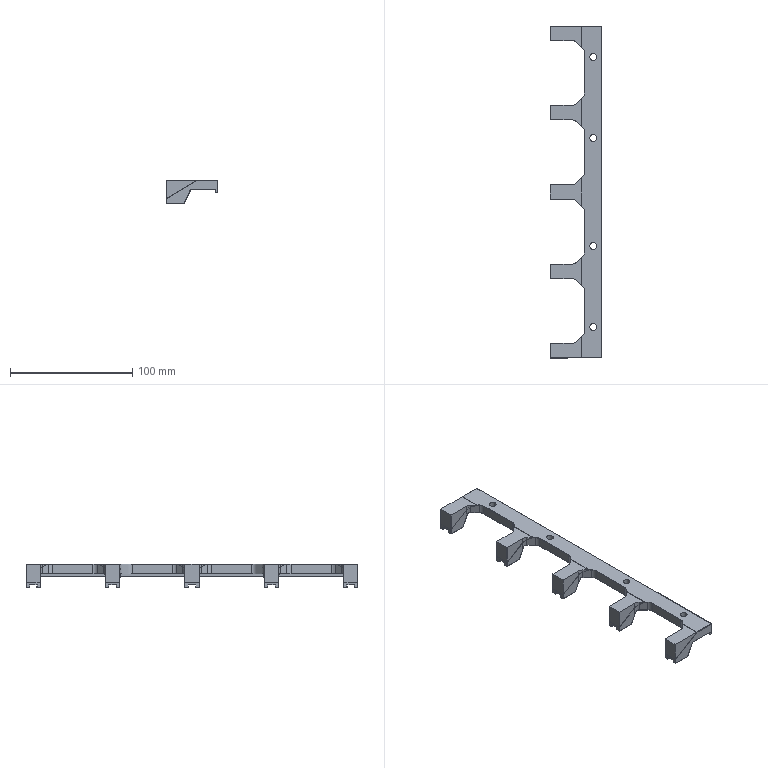CAM job | NX | 3+2 milling, drilling | part box 42 x 271.8 x 19 mm | stock box 45 x 277 x 25 mm
Tools:
number,name,description,diameter,corner_radius,flute_length,length,flutes
4,D4,平底铣刀-粗,4.0,0.0,25.0,75.0,2
6,D6,平底铣刀-粗,6.0,0.0,25.0,75.0,2
9,D10,平底铣刀-粗,10.0,0.0,35.0,75.0,2
7,D6-J,平底铣刀-精,6.0,0.0,25.0,75.0,2
10,D10-J,平底铣刀-精,10.0,0.0,35.0,75.0,2
18,D6R0.5,圆鼻刀-粗,6.0,0.5,50.0,75.0,2
1,D80R0.8飞刀,圆鼻刀-粗,80.0,0.8,50.0,75.0,2
2,D6倒角刀,倒角刀,6.0,0.0,3.0,25.0,2
17,钻头5.5,Twist Drill 5 mm,5.5,0.0,52.0,54.0,2
Operations:
program,operation,operation_type,tool,method,geometry_group,spindle_rpm,surface_speed,feed_per_tooth,feed_cut,feed_plunge,cut_length_mm,path_length_mm,cut_time_min,machine_time_min
C,型腔铣开粗-中_COPY_1,CavityMilling,D6,分层开粗-切深K-步距G,W-C,8000.0,150.796,0.1875,3000.0,100.0,19481.465,24446.704,6.494,7.228
C,等高精光往复爬面_COPY_1_COPY,ZLevelMilling,D6R0.5,等高爬面-切深K-步距G,W-C,7000.0,131.947,0.2857,4000.0,100.0,36709.228,37755.282,9.177,9.282
B,动态开粗D10_COPY_1,CavityMilling,D10,动态开粗-切深K-步距K,W-B,8000.0,251.32,0.25,4000.0,100.0,27133.852,27169.652,6.784,6.787
B,型腔铣开粗-中_COPY,CavityMilling,D10,分层开粗-切深K-步距G,W-B,8000.0,251.32,0.25,4000.0,100.0,20003.603,20348.798,5.001,5.05
B,底壁铣分层开粗-中_COPY,VolumeBased25DMillingOperation,D4,分层开粗-切深K-步距G,W-B,8000.0,100.528,0.125,2000.0,100.0,2370.316,2705.264,1.185,1.219
B,平面去毛刺6X45L_COPY,SurfaceContour,D6倒角刀,爬面_倒角-切深0-步距G,W-B,6500.0,122.519,0.1154,1500.0,100.0,1332.351,3197.122,0.8882,1.075
B,等高精光往复爬面_COPY,ZLevelMilling,D6R0.5,等高爬面-切深K-步距G,W-B,7000.0,131.947,0.2857,4000.0,100.0,12801.608,13764.402,3.2,3.297
B,底壁铣精光底面-中_COPY,VolumeBased25DMillingOperation,D6-J,精光步距切深关,W-B,7000.0,175.0,0.0536,1500.0,100.0,577.774,939.299,0.3852,0.4213
B,底壁铣精光侧面-中-选底面_COPY,VolumeBased25DMillingOperation,D6-J,侧刃精光-切深K-步距G,W-B,8000.0,150.792,0.0625,1000.0,100.0,290.569,601.588,0.2906,0.3217
B,底壁铣精光底面-中_COPY_2,VolumeBased25DMillingOperation,D6-J,精光步距切深关,W-B,7000.0,175.0,0.0536,1500.0,100.0,563.137,610.237,0.3754,0.3801
B,底壁铣精光底面-中_COPY_1,VolumeBased25DMillingOperation,D6-J,精光步距切深关,W-B,8000.0,150.792,0.0625,1000.0,100.0,1319.547,1370.647,1.319,1.325
B,底壁铣精光侧面-中-选底面_COPY_1,VolumeBased25DMillingOperation,D6-J,侧刃精光-切深K-步距G,W-B,8000.0,150.792,0.0625,1000.0,100.0,422.395,642.365,0.4224,0.4444
A,顶面,FaceMilling,D80R0.8飞刀,侧刃精光-切深K-步距G,W-A,5000.0,1256.637,0.1,1000.0,100.0,365.8,401.8,0.3658,0.3694
A,动态开粗D10_COPY,CavityMilling,D10,动态开粗-切深K-步距K,W-A,8000.0,251.32,0.25,4000.0,100.0,11667.014,11742.014,2.917,2.924
A,打点-深0.8,Operation,D6倒角刀,NONE,W-A,8000.0,150.796,0.0312,500.0,90.0,7.2,278.621,0.0144,0.0415
A,通孔-5-6,Operation,钻头5.5,NONE,W-A,3000.0,51.836,0.0417,250.0,90.0,49.609,363.44,0.1984,0.2298
A,仅选体,SurfaceContour,D6倒角刀,METHOD,W-A,8000.0,150.796,0.1875,3000.0,100.0,826.183,861.985,0.2754,0.279
A,铣倒角_1,PlanarMilling,D6倒角刀,METHOD,W-A,8000.0,150.796,0.0312,500.0,100.0,78.753,469.868,0.1575,0.1966
A,外形半精_2,VolumeBased25DMillingOperation,D10-J,METHOD,W-A,8000.0,251.327,0.0625,1000.0,100.0,845.284,923.284,0.8453,0.8531